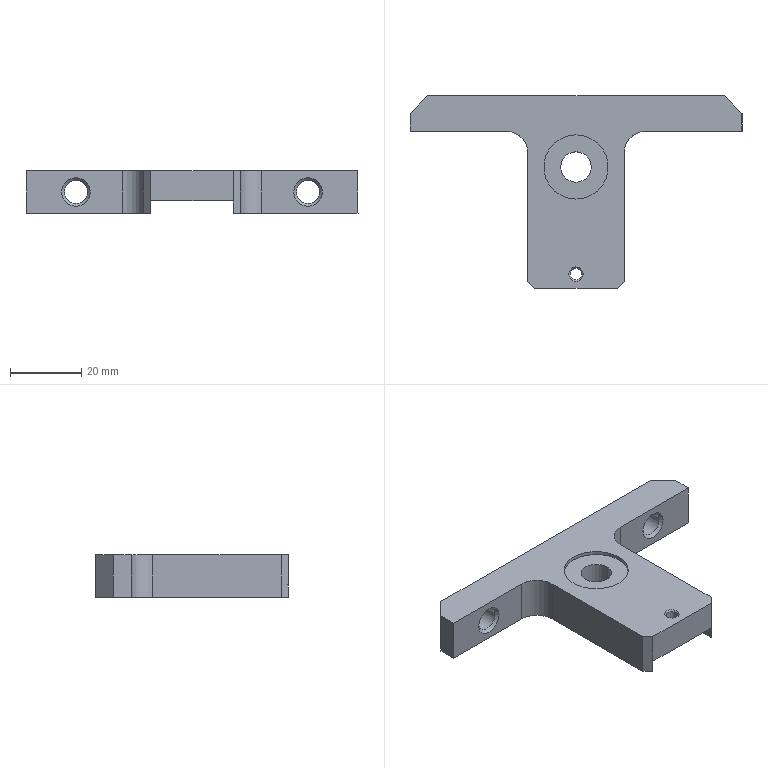Part | STEP file | 1 solid | 38 faces | box 93 x 54 x 12 mm | volume 19290 mm3 | plane 19 | cone 10 | cylinder 9 | commonest cylinder face diameters 3.242 x3 6.4 x2 12 x2 8.5 x1 18 x1